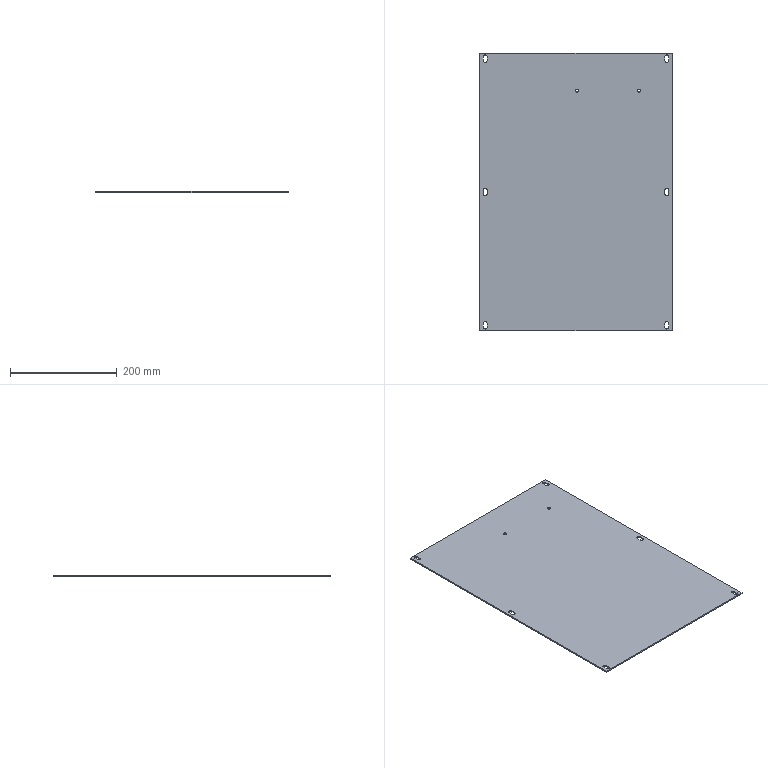Part | SolidWorks | features FlatPattern 1, SMBaseFlange 1, SheetMetal 1 | 1 solid | 34 faces | box 360 x 520 x 2.5 mm | volume 466582 mm3 | plane 18 | cylinder 16 | commonest cylinder face diameters 7 x12 5.2 x4
STEP:
#1=CARTESIAN_POINT('',(-180.6,450.,2.5));
#2=VERTEX_POINT('',#1);
#3=CARTESIAN_POINT('',(-175.4,450.,2.5));
#4=VERTEX_POINT('',#3);
#5=CARTESIAN_POINT('',(-178.,450.,2.5));
#6=DIRECTION('',(0.,0.,1.));
#7=DIRECTION('',(1.,0.,0.));
#8=AXIS2_PLACEMENT_3D('',#5,#6,#7);
#9=CIRCLE('',#8,2.6);
#10=EDGE_CURVE('',#2,#4,#9,.T.);
#11=ORIENTED_EDGE('',*,*,#10,.T.);
#12=CARTESIAN_POINT('',(-175.4,450.,0.));
#13=VERTEX_POINT('',#12);
#14=CARTESIAN_POINT('',(-175.4,450.,2.5));
#15=DIRECTION('',(0.,0.,-1.));
#16=VECTOR('',#15,1000.);
#17=LINE('',#14,#16);
#18=EDGE_CURVE('',#4,#13,#17,.T.);
#19=ORIENTED_EDGE('',*,*,#18,.T.);
#20=CARTESIAN_POINT('',(-180.6,450.,0.));
#21=VERTEX_POINT('',#20);
#22=CARTESIAN_POINT('',(-178.,450.,0.));
#23=DIRECTION('',(0.,0.,1.));
#24=DIRECTION('',(1.,0.,0.));
#25=AXIS2_PLACEMENT_3D('',#22,#23,#24);
#26=CIRCLE('',#25,2.6);
#27=EDGE_CURVE('',#21,#13,#26,.T.);
#28=ORIENTED_EDGE('',*,*,#27,.F.);
#29=CARTESIAN_POINT('',(-180.6,450.,2.5));
#30=DIRECTION('',(0.,0.,-1.));
#31=VECTOR('',#30,1000.);
#32=LINE('',#29,#31);
#33=EDGE_CURVE('',#2,#21,#32,.T.);
#34=ORIENTED_EDGE('',*,*,#33,.F.);
#35=EDGE_LOOP('',(#11,#19,#28,#34));
#36=FACE_OUTER_BOUND('',#35,.T.);
#37=CARTESIAN_POINT('',(-178.,450.,2.5));
#38=DIRECTION('',(0.,0.,-1.));
#39=DIRECTION('',(-1.,0.,0.));
#40=AXIS2_PLACEMENT_3D('',#37,#38,#39);
#41=CYLINDRICAL_SURFACE('',#40,2.6);
#42=ADVANCED_FACE('',(#36),#41,.F.);
#43=CARTESIAN_POINT('',(-64.6,450.,2.5));
#44=VERTEX_POINT('',#43);
#45=CARTESIAN_POINT('',(-59.4,450.,2.5));
#46=VERTEX_POINT('',#45);
#47=CARTESIAN_POINT('',(-62.,450.,2.5));
#48=DIRECTION('',(0.,0.,1.));
#49=DIRECTION('',(1.,0.,0.));
#50=AXIS2_PLACEMENT_3D('',#47,#48,#49);
#51=CIRCLE('',#50,2.6);
#52=EDGE_CURVE('',#44,#46,#51,.T.);
#53=ORIENTED_EDGE('',*,*,#52,.T.);
#54=CARTESIAN_POINT('',(-59.4,450.,0.));
#55=VERTEX_POINT('',#54);
#56=CARTESIAN_POINT('',(-59.4,450.,2.5));
#57=DIRECTION('',(0.,0.,-1.));
#58=VECTOR('',#57,1000.);
#59=LINE('',#56,#58);
#60=EDGE_CURVE('',#46,#55,#59,.T.);
#61=ORIENTED_EDGE('',*,*,#60,.T.);
#62=CARTESIAN_POINT('',(-64.6,450.,0.));
#63=VERTEX_POINT('',#62);
#64=CARTESIAN_POINT('',(-62.,450.,0.));
#65=DIRECTION('',(0.,0.,1.));
#66=DIRECTION('',(1.,0.,0.));
#67=AXIS2_PLACEMENT_3D('',#64,#65,#66);
#68=CIRCLE('',#67,2.6);
#69=EDGE_CURVE('',#63,#55,#68,.T.);
#70=ORIENTED_EDGE('',*,*,#69,.F.);
#71=CARTESIAN_POINT('',(-64.6,450.,2.5));
#72=DIRECTION('',(0.,0.,-1.));
#73=VECTOR('',#72,1000.);
#74=LINE('',#71,#73);
#75=EDGE_CURVE('',#44,#63,#74,.T.);
#76=ORIENTED_EDGE('',*,*,#75,.F.);
#77=EDGE_LOOP('',(#53,#61,#70,#76));
#78=FACE_OUTER_BOUND('',#77,.T.);
#79=CARTESIAN_POINT('',(-62.,450.,2.5));
#80=DIRECTION('',(0.,0.,-1.));
#81=DIRECTION('',(-1.,0.,0.));
#82=AXIS2_PLACEMENT_3D('',#79,#80,#81);
#83=CYLINDRICAL_SURFACE('',#82,2.6);
#84=ADVANCED_FACE('',(#78),#83,.F.);
#85=CARTESIAN_POINT('',(-13.5,513.5,2.5));
#86=VERTEX_POINT('',#85);
#87=CARTESIAN_POINT('',(-13.5,506.5,2.5));
#88=VERTEX_POINT('',#87);
#89=CARTESIAN_POINT('',(-13.5,513.5,2.5));
#90=DIRECTION('',(0.,-1.,0.));
#91=VECTOR('',#90,1000.);
#92=LINE('',#89,#91);
#93=EDGE_CURVE('',#86,#88,#92,.T.);
#94=ORIENTED_EDGE('',*,*,#93,.F.);
#95=CARTESIAN_POINT('',(-6.5,513.5,2.5));
#96=VERTEX_POINT('',#95);
#97=CARTESIAN_POINT('',(-10.,513.5,2.5));
#98=DIRECTION('',(0.,0.,1.));
#99=DIRECTION('',(-1.,0.,0.));
#100=AXIS2_PLACEMENT_3D('',#97,#98,#99);
#101=CIRCLE('',#100,3.5);
#102=EDGE_CURVE('',#96,#86,#101,.T.);
#103=ORIENTED_EDGE('',*,*,#102,.F.);
#104=CARTESIAN_POINT('',(-6.5,506.5,2.5));
#105=VERTEX_POINT('',#104);
#106=CARTESIAN_POINT('',(-6.5,513.5,2.5));
#107=DIRECTION('',(0.,1.,0.));
#108=VECTOR('',#107,1000.);
#109=LINE('',#106,#108);
#110=EDGE_CURVE('',#105,#96,#109,.T.);
#111=ORIENTED_EDGE('',*,*,#110,.F.);
#112=CARTESIAN_POINT('',(-10.,506.5,2.5));
#113=DIRECTION('',(0.,0.,1.));
#114=DIRECTION('',(-1.,0.,0.));
#115=AXIS2_PLACEMENT_3D('',#112,#113,#114);
#116=CIRCLE('',#115,3.5);
#117=EDGE_CURVE('',#88,#105,#116,.T.);
#118=ORIENTED_EDGE('',*,*,#117,.F.);
#119=EDGE_LOOP('',(#94,#103,#111,#118));
#120=FACE_BOUND('',#119,.T.);
#121=CARTESIAN_POINT('',(-13.5,263.5,2.5));
#122=VERTEX_POINT('',#121);
#123=CARTESIAN_POINT('',(-13.5,256.5,2.5));
#124=VERTEX_POINT('',#123);
#125=CARTESIAN_POINT('',(-13.5,263.5,2.5));
#126=DIRECTION('',(0.,-1.,0.));
#127=VECTOR('',#126,1000.);
#128=LINE('',#125,#127);
#129=EDGE_CURVE('',#122,#124,#128,.T.);
#130=ORIENTED_EDGE('',*,*,#129,.F.);
#131=CARTESIAN_POINT('',(-6.5,263.5,2.5));
#132=VERTEX_POINT('',#131);
#133=CARTESIAN_POINT('',(-10.,263.5,2.5));
#134=DIRECTION('',(0.,0.,1.));
#135=DIRECTION('',(-1.,0.,0.));
#136=AXIS2_PLACEMENT_3D('',#133,#134,#135);
#137=CIRCLE('',#136,3.5);
#138=EDGE_CURVE('',#132,#122,#137,.T.);
#139=ORIENTED_EDGE('',*,*,#138,.F.);
#140=CARTESIAN_POINT('',(-6.5,256.5,2.5));
#141=VERTEX_POINT('',#140);
#142=CARTESIAN_POINT('',(-6.5,263.5,2.5));
#143=DIRECTION('',(0.,1.,0.));
#144=VECTOR('',#143,1000.);
#145=LINE('',#142,#144);
#146=EDGE_CURVE('',#141,#132,#145,.T.);
#147=ORIENTED_EDGE('',*,*,#146,.F.);
#148=CARTESIAN_POINT('',(-10.,256.5,2.5));
#149=DIRECTION('',(0.,0.,1.));
#150=DIRECTION('',(-1.,0.,0.));
#151=AXIS2_PLACEMENT_3D('',#148,#149,#150);
#152=CIRCLE('',#151,3.5);
#153=EDGE_CURVE('',#124,#141,#152,.T.);
#154=ORIENTED_EDGE('',*,*,#153,.F.);
#155=EDGE_LOOP('',(#130,#139,#147,#154));
#156=FACE_BOUND('',#155,.T.);
#157=CARTESIAN_POINT('',(-13.5,13.5,2.5));
#158=VERTEX_POINT('',#157);
#159=CARTESIAN_POINT('',(-13.5,6.5,2.5));
#160=VERTEX_POINT('',#159);
#161=CARTESIAN_POINT('',(-13.5,13.5,2.5));
#162=DIRECTION('',(0.,-1.,0.));
#163=VECTOR('',#162,1000.);
#164=LINE('',#161,#163);
#165=EDGE_CURVE('',#158,#160,#164,.T.);
#166=ORIENTED_EDGE('',*,*,#165,.F.);
#167=CARTESIAN_POINT('',(-6.5,13.5,2.5));
#168=VERTEX_POINT('',#167);
#169=CARTESIAN_POINT('',(-10.,13.5,2.5));
#170=DIRECTION('',(0.,0.,1.));
#171=DIRECTION('',(-1.,0.,0.));
#172=AXIS2_PLACEMENT_3D('',#169,#170,#171);
#173=CIRCLE('',#172,3.5);
#174=EDGE_CURVE('',#168,#158,#173,.T.);
#175=ORIENTED_EDGE('',*,*,#174,.F.);
#176=CARTESIAN_POINT('',(-6.5,6.5,2.5));
#177=VERTEX_POINT('',#176);
#178=CARTESIAN_POINT('',(-6.5,13.5,2.5));
#179=DIRECTION('',(0.,1.,0.));
#180=VECTOR('',#179,1000.);
#181=LINE('',#178,#180);
#182=EDGE_CURVE('',#177,#168,#181,.T.);
#183=ORIENTED_EDGE('',*,*,#182,.F.);
#184=CARTESIAN_POINT('',(-10.,6.5,2.5));
#185=DIRECTION('',(0.,0.,1.));
#186=DIRECTION('',(-1.,0.,0.));
#187=AXIS2_PLACEMENT_3D('',#184,#185,#186);
#188=CIRCLE('',#187,3.5);
#189=EDGE_CURVE('',#160,#177,#188,.T.);
#190=ORIENTED_EDGE('',*,*,#189,.F.);
#191=EDGE_LOOP('',(#166,#175,#183,#190));
#192=FACE_BOUND('',#191,.T.);
#193=CARTESIAN_POINT('',(-353.5,13.5,2.5));
#194=VERTEX_POINT('',#193);
#195=CARTESIAN_POINT('',(-353.5,6.5,2.5));
#196=VERTEX_POINT('',#195);
#197=CARTESIAN_POINT('',(-353.5,13.5,2.5));
#198=DIRECTION('',(0.,-1.,0.));
#199=VECTOR('',#198,1000.);
#200=LINE('',#197,#199);
#201=EDGE_CURVE('',#194,#196,#200,.T.);
#202=ORIENTED_EDGE('',*,*,#201,.F.);
#203=CARTESIAN_POINT('',(-346.5,13.5,2.5));
#204=VERTEX_POINT('',#203);
#205=CARTESIAN_POINT('',(-350.,13.5,2.5));
#206=DIRECTION('',(0.,0.,1.));
#207=DIRECTION('',(-1.,0.,0.));
#208=AXIS2_PLACEMENT_3D('',#205,#206,#207);
#209=CIRCLE('',#208,3.5);
#210=EDGE_CURVE('',#204,#194,#209,.T.);
#211=ORIENTED_EDGE('',*,*,#210,.F.);
#212=CARTESIAN_POINT('',(-346.5,6.5,2.5));
#213=VERTEX_POINT('',#212);
#214=CARTESIAN_POINT('',(-346.5,13.5,2.5));
#215=DIRECTION('',(0.,1.,0.));
#216=VECTOR('',#215,1000.);
#217=LINE('',#214,#216);
#218=EDGE_CURVE('',#213,#204,#217,.T.);
#219=ORIENTED_EDGE('',*,*,#218,.F.);
#220=CARTESIAN_POINT('',(-350.,6.5,2.5));
#221=DIRECTION('',(0.,0.,1.));
#222=DIRECTION('',(-1.,0.,0.));
#223=AXIS2_PLACEMENT_3D('',#220,#221,#222);
#224=CIRCLE('',#223,3.5);
#225=EDGE_CURVE('',#196,#213,#224,.T.);
#226=ORIENTED_EDGE('',*,*,#225,.F.);
#227=EDGE_LOOP('',(#202,#211,#219,#226));
#228=FACE_BOUND('',#227,.T.);
#229=CARTESIAN_POINT('',(0.,0.,2.5));
#230=VERTEX_POINT('',#229);
#231=CARTESIAN_POINT('',(0.,520.,2.5));
#232=VERTEX_POINT('',#231);
#233=CARTESIAN_POINT('',(0.,0.,2.5));
#234=DIRECTION('',(0.,1.,0.));
#235=VECTOR('',#234,1000.);
#236=LINE('',#233,#235);
#237=EDGE_CURVE('',#230,#232,#236,.T.);
#238=ORIENTED_EDGE('',*,*,#237,.T.);
#239=CARTESIAN_POINT('',(-360.,520.,2.5));
#240=VERTEX_POINT('',#239);
#241=CARTESIAN_POINT('',(0.,520.,2.5));
#242=DIRECTION('',(-1.,0.,0.));
#243=VECTOR('',#242,1000.);
#244=LINE('',#241,#243);
#245=EDGE_CURVE('',#232,#240,#244,.T.);
#246=ORIENTED_EDGE('',*,*,#245,.T.);
#247=CARTESIAN_POINT('',(-360.,0.,2.5));
#248=VERTEX_POINT('',#247);
#249=CARTESIAN_POINT('',(-360.,0.,2.5));
#250=DIRECTION('',(0.,-1.,0.));
#251=VECTOR('',#250,1000.);
#252=LINE('',#249,#251);
#253=EDGE_CURVE('',#240,#248,#252,.T.);
#254=ORIENTED_EDGE('',*,*,#253,.T.);
#255=CARTESIAN_POINT('',(0.,0.,2.5));
#256=DIRECTION('',(1.,0.,0.));
#257=VECTOR('',#256,1000.);
#258=LINE('',#255,#257);
#259=EDGE_CURVE('',#248,#230,#258,.T.);
#260=ORIENTED_EDGE('',*,*,#259,.T.);
#261=EDGE_LOOP('',(#238,#246,#254,#260));
#262=FACE_OUTER_BOUND('',#261,.T.);
#263=ORIENTED_EDGE('',*,*,#52,.F.);
#264=CARTESIAN_POINT('',(-62.,450.,2.5));
#265=DIRECTION('',(0.,0.,1.));
#266=DIRECTION('',(1.,0.,0.));
#267=AXIS2_PLACEMENT_3D('',#264,#265,#266);
#268=CIRCLE('',#267,2.6);
#269=EDGE_CURVE('',#46,#44,#268,.T.);
#270=ORIENTED_EDGE('',*,*,#269,.F.);
#271=EDGE_LOOP('',(#263,#270));
#272=FACE_BOUND('',#271,.T.);
#273=CARTESIAN_POINT('',(-353.5,263.5,2.5));
#274=VERTEX_POINT('',#273);
#275=CARTESIAN_POINT('',(-353.5,256.5,2.5));
#276=VERTEX_POINT('',#275);
#277=CARTESIAN_POINT('',(-353.5,263.5,2.5));
#278=DIRECTION('',(0.,-1.,0.));
#279=VECTOR('',#278,1000.);
#280=LINE('',#277,#279);
#281=EDGE_CURVE('',#274,#276,#280,.T.);
#282=ORIENTED_EDGE('',*,*,#281,.F.);
#283=CARTESIAN_POINT('',(-346.5,263.5,2.5));
#284=VERTEX_POINT('',#283);
#285=CARTESIAN_POINT('',(-350.,263.5,2.5));
#286=DIRECTION('',(0.,0.,1.));
#287=DIRECTION('',(-1.,0.,0.));
#288=AXIS2_PLACEMENT_3D('',#285,#286,#287);
#289=CIRCLE('',#288,3.5);
#290=EDGE_CURVE('',#284,#274,#289,.T.);
#291=ORIENTED_EDGE('',*,*,#290,.F.);
#292=CARTESIAN_POINT('',(-346.5,256.5,2.5));
#293=VERTEX_POINT('',#292);
#294=CARTESIAN_POINT('',(-346.5,263.5,2.5));
#295=DIRECTION('',(0.,1.,0.));
#296=VECTOR('',#295,1000.);
#297=LINE('',#294,#296);
#298=EDGE_CURVE('',#293,#284,#297,.T.);
#299=ORIENTED_EDGE('',*,*,#298,.F.);
#300=CARTESIAN_POINT('',(-350.,256.5,2.5));
#301=DIRECTION('',(0.,0.,1.));
#302=DIRECTION('',(-1.,0.,0.));
#303=AXIS2_PLACEMENT_3D('',#300,#301,#302);
#304=CIRCLE('',#303,3.5);
#305=EDGE_CURVE('',#276,#293,#304,.T.);
#306=ORIENTED_EDGE('',*,*,#305,.F.);
#307=EDGE_LOOP('',(#282,#291,#299,#306));
#308=FACE_BOUND('',#307,.T.);
#309=CARTESIAN_POINT('',(-353.5,513.5,2.5));
#310=VERTEX_POINT('',#309);
#311=CARTESIAN_POINT('',(-353.5,506.5,2.5));
#312=VERTEX_POINT('',#311);
#313=CARTESIAN_POINT('',(-353.5,513.5,2.5));
#314=DIRECTION('',(0.,-1.,0.));
#315=VECTOR('',#314,1000.);
#316=LINE('',#313,#315);
#317=EDGE_CURVE('',#310,#312,#316,.T.);
#318=ORIENTED_EDGE('',*,*,#317,.F.);
#319=CARTESIAN_POINT('',(-346.5,513.5,2.5));
#320=VERTEX_POINT('',#319);
#321=CARTESIAN_POINT('',(-350.,513.5,2.5));
#322=DIRECTION('',(0.,0.,1.));
#323=DIRECTION('',(-1.,0.,0.));
#324=AXIS2_PLACEMENT_3D('',#321,#322,#323);
#325=CIRCLE('',#324,3.5);
#326=EDGE_CURVE('',#320,#310,#325,.T.);
#327=ORIENTED_EDGE('',*,*,#326,.F.);
#328=CARTESIAN_POINT('',(-346.5,506.5,2.5));
#329=VERTEX_POINT('',#328);
#330=CARTESIAN_POINT('',(-346.5,513.5,2.5));
#331=DIRECTION('',(0.,1.,0.));
#332=VECTOR('',#331,1000.);
#333=LINE('',#330,#332);
#334=EDGE_CURVE('',#329,#320,#333,.T.);
#335=ORIENTED_EDGE('',*,*,#334,.F.);
#336=CARTESIAN_POINT('',(-350.,506.5,2.5));
#337=DIRECTION('',(0.,0.,1.));
#338=DIRECTION('',(-1.,0.,0.));
#339=AXIS2_PLACEMENT_3D('',#336,#337,#338);
#340=CIRCLE('',#339,3.5);
#341=EDGE_CURVE('',#312,#329,#340,.T.);
#342=ORIENTED_EDGE('',*,*,#341,.F.);
#343=EDGE_LOOP('',(#318,#327,#335,#342));
#344=FACE_BOUND('',#343,.T.);
#345=ORIENTED_EDGE('',*,*,#10,.F.);
#346=CARTESIAN_POINT('',(-178.,450.,2.5));
#347=DIRECTION('',(0.,0.,1.));
#348=DIRECTION('',(1.,0.,0.));
#349=AXIS2_PLACEMENT_3D('',#346,#347,#348);
#350=CIRCLE('',#349,2.6);
#351=EDGE_CURVE('',#4,#2,#350,.T.);
#352=ORIENTED_EDGE('',*,*,#351,.F.);
#353=EDGE_LOOP('',(#345,#352));
#354=FACE_BOUND('',#353,.T.);
#355=CARTESIAN_POINT('',(0.,0.,2.5));
#356=DIRECTION('',(0.,0.,1.));
#357=DIRECTION('',(1.,0.,0.));
#358=AXIS2_PLACEMENT_3D('',#355,#356,#357);
#359=PLANE('',#358);
#360=ADVANCED_FACE('',(#120,#156,#192,#228,#262,#272,#308,#344,#354),#359,.T.);
#361=CARTESIAN_POINT('',(-6.5,513.5,0.));
#362=VERTEX_POINT('',#361);
#363=CARTESIAN_POINT('',(-13.5,513.5,0.));
#364=VERTEX_POINT('',#363);
#365=CARTESIAN_POINT('',(-10.,513.5,0.));
#366=DIRECTION('',(0.,0.,1.));
#367=DIRECTION('',(-1.,0.,0.));
#368=AXIS2_PLACEMENT_3D('',#365,#366,#367);
#369=CIRCLE('',#368,3.5);
#370=EDGE_CURVE('',#362,#364,#369,.T.);
#371=ORIENTED_EDGE('',*,*,#370,.T.);
#372=CARTESIAN_POINT('',(-13.5,506.5,0.));
#373=VERTEX_POINT('',#372);
#374=CARTESIAN_POINT('',(-13.5,513.5,0.));
#375=DIRECTION('',(0.,-1.,0.));
#376=VECTOR('',#375,1000.);
#377=LINE('',#374,#376);
#378=EDGE_CURVE('',#364,#373,#377,.T.);
#379=ORIENTED_EDGE('',*,*,#378,.T.);
#380=CARTESIAN_POINT('',(-6.5,506.5,0.));
#381=VERTEX_POINT('',#380);
#382=CARTESIAN_POINT('',(-10.,506.5,0.));
#383=DIRECTION('',(0.,0.,1.));
#384=DIRECTION('',(-1.,0.,0.));
#385=AXIS2_PLACEMENT_3D('',#382,#383,#384);
#386=CIRCLE('',#385,3.5);
#387=EDGE_CURVE('',#373,#381,#386,.T.);
#388=ORIENTED_EDGE('',*,*,#387,.T.);
#389=CARTESIAN_POINT('',(-6.5,513.5,0.));
#390=DIRECTION('',(0.,1.,0.));
#391=VECTOR('',#390,1000.);
#392=LINE('',#389,#391);
#393=EDGE_CURVE('',#381,#362,#392,.T.);
#394=ORIENTED_EDGE('',*,*,#393,.T.);
#395=EDGE_LOOP('',(#371,#379,#388,#394));
#396=FACE_BOUND('',#395,.T.);
#397=CARTESIAN_POINT('',(-6.5,263.5,0.));
#398=VERTEX_POINT('',#397);
#399=CARTESIAN_POINT('',(-13.5,263.5,0.));
#400=VERTEX_POINT('',#399);
#401=CARTESIAN_POINT('',(-10.,263.5,0.));
#402=DIRECTION('',(0.,0.,1.));
#403=DIRECTION('',(-1.,0.,0.));
#404=AXIS2_PLACEMENT_3D('',#401,#402,#403);
#405=CIRCLE('',#404,3.5);
#406=EDGE_CURVE('',#398,#400,#405,.T.);
#407=ORIENTED_EDGE('',*,*,#406,.T.);
#408=CARTESIAN_POINT('',(-13.5,256.5,0.));
#409=VERTEX_POINT('',#408);
#410=CARTESIAN_POINT('',(-13.5,263.5,0.));
#411=DIRECTION('',(0.,-1.,0.));
#412=VECTOR('',#411,1000.);
#413=LINE('',#410,#412);
#414=EDGE_CURVE('',#400,#409,#413,.T.);
#415=ORIENTED_EDGE('',*,*,#414,.T.);
#416=CARTESIAN_POINT('',(-6.5,256.5,0.));
#417=VERTEX_POINT('',#416);
#418=CARTESIAN_POINT('',(-10.,256.5,0.));
#419=DIRECTION('',(0.,0.,1.));
#420=DIRECTION('',(-1.,0.,0.));
#421=AXIS2_PLACEMENT_3D('',#418,#419,#420);
#422=CIRCLE('',#421,3.5);
#423=EDGE_CURVE('',#409,#417,#422,.T.);
#424=ORIENTED_EDGE('',*,*,#423,.T.);
#425=CARTESIAN_POINT('',(-6.5,263.5,0.));
#426=DIRECTION('',(0.,1.,0.));
#427=VECTOR('',#426,1000.);
#428=LINE('',#425,#427);
#429=EDGE_CURVE('',#417,#398,#428,.T.);
#430=ORIENTED_EDGE('',*,*,#429,.T.);
#431=EDGE_LOOP('',(#407,#415,#424,#430));
#432=FACE_BOUND('',#431,.T.);
#433=CARTESIAN_POINT('',(-6.5,13.5,0.));
#434=VERTEX_POINT('',#433);
#435=CARTESIAN_POINT('',(-13.5,13.5,0.));
#436=VERTEX_POINT('',#435);
#437=CARTESIAN_POINT('',(-10.,13.5,0.));
#438=DIRECTION('',(0.,0.,1.));
#439=DIRECTION('',(-1.,0.,0.));
#440=AXIS2_PLACEMENT_3D('',#437,#438,#439);
#441=CIRCLE('',#440,3.5);
#442=EDGE_CURVE('',#434,#436,#441,.T.);
#443=ORIENTED_EDGE('',*,*,#442,.T.);
#444=CARTESIAN_POINT('',(-13.5,6.5,0.));
#445=VERTEX_POINT('',#444);
#446=CARTESIAN_POINT('',(-13.5,13.5,0.));
#447=DIRECTION('',(0.,-1.,0.));
#448=VECTOR('',#447,1000.);
#449=LINE('',#446,#448);
#450=EDGE_CURVE('',#436,#445,#449,.T.);
#451=ORIENTED_EDGE('',*,*,#450,.T.);
#452=CARTESIAN_POINT('',(-6.5,6.5,0.));
#453=VERTEX_POINT('',#452);
#454=CARTESIAN_POINT('',(-10.,6.5,0.));
#455=DIRECTION('',(0.,0.,1.));
#456=DIRECTION('',(-1.,0.,0.));
#457=AXIS2_PLACEMENT_3D('',#454,#455,#456);
#458=CIRCLE('',#457,3.5);
#459=EDGE_CURVE('',#445,#453,#458,.T.);
#460=ORIENTED_EDGE('',*,*,#459,.T.);
#461=CARTESIAN_POINT('',(-6.5,13.5,0.));
#462=DIRECTION('',(0.,1.,0.));
#463=VECTOR('',#462,1000.);
#464=LINE('',#461,#463);
#465=EDGE_CURVE('',#453,#434,#464,.T.);
#466=ORIENTED_EDGE('',*,*,#465,.T.);
#467=EDGE_LOOP('',(#443,#451,#460,#466));
#468=FACE_BOUND('',#467,.T.);
#469=CARTESIAN_POINT('',(-346.5,13.5,0.));
#470=VERTEX_POINT('',#469);
#471=CARTESIAN_POINT('',(-353.5,13.5,0.));
#472=VERTEX_POINT('',#471);
#473=CARTESIAN_POINT('',(-350.,13.5,0.));
#474=DIRECTION('',(0.,0.,1.));
#475=DIRECTION('',(-1.,0.,0.));
#476=AXIS2_PLACEMENT_3D('',#473,#474,#475);
#477=CIRCLE('',#476,3.5);
#478=EDGE_CURVE('',#470,#472,#477,.T.);
#479=ORIENTED_EDGE('',*,*,#478,.T.);
#480=CARTESIAN_POINT('',(-353.5,6.5,0.));
#481=VERTEX_POINT('',#480);
#482=CARTESIAN_POINT('',(-353.5,13.5,0.));
#483=DIRECTION('',(0.,-1.,0.));
#484=VECTOR('',#483,1000.);
#485=LINE('',#482,#484);
#486=EDGE_CURVE('',#472,#481,#485,.T.);
#487=ORIENTED_EDGE('',*,*,#486,.T.);
#488=CARTESIAN_POINT('',(-346.5,6.5,0.));
#489=VERTEX_POINT('',#488);
#490=CARTESIAN_POINT('',(-350.,6.5,0.));
#491=DIRECTION('',(0.,0.,1.));
#492=DIRECTION('',(-1.,0.,0.));
#493=AXIS2_PLACEMENT_3D('',#490,#491,#492);
#494=CIRCLE('',#493,3.5);
#495=EDGE_CURVE('',#481,#489,#494,.T.);
#496=ORIENTED_EDGE('',*,*,#495,.T.);
#497=CARTESIAN_POINT('',(-346.5,13.5,0.));
#498=DIRECTION('',(0.,1.,0.));
#499=VECTOR('',#498,1000.);
#500=LINE('',#497,#499);
#501=EDGE_CURVE('',#489,#470,#500,.T.);
#502=ORIENTED_EDGE('',*,*,#501,.T.);
#503=EDGE_LOOP('',(#479,#487,#496,#502));
#504=FACE_BOUND('',#503,.T.);
#505=CARTESIAN_POINT('',(0.,0.,0.));
#506=VERTEX_POINT('',#505);
#507=CARTESIAN_POINT('',(0.,520.,0.));
#508=VERTEX_POINT('',#507);
#509=CARTESIAN_POINT('',(0.,0.,0.));
#510=DIRECTION('',(0.,1.,0.));
#511=VECTOR('',#510,1000.);
#512=LINE('',#509,#511);
#513=EDGE_CURVE('',#506,#508,#512,.T.);
#514=ORIENTED_EDGE('',*,*,#513,.F.);
#515=CARTESIAN_POINT('',(-360.,0.,0.));
#516=VERTEX_POINT('',#515);
#517=CARTESIAN_POINT('',(0.,0.,0.));
#518=DIRECTION('',(1.,0.,0.));
#519=VECTOR('',#518,1000.);
#520=LINE('',#517,#519);
#521=EDGE_CURVE('',#516,#506,#520,.T.);
#522=ORIENTED_EDGE('',*,*,#521,.F.);
#523=CARTESIAN_POINT('',(-360.,520.,0.));
#524=VERTEX_POINT('',#523);
#525=CARTESIAN_POINT('',(-360.,0.,0.));
#526=DIRECTION('',(0.,-1.,0.));
#527=VECTOR('',#526,1000.);
#528=LINE('',#525,#527);
#529=EDGE_CURVE('',#524,#516,#528,.T.);
#530=ORIENTED_EDGE('',*,*,#529,.F.);
#531=CARTESIAN_POINT('',(0.,520.,0.));
#532=DIRECTION('',(-1.,0.,0.));
#533=VECTOR('',#532,1000.);
#534=LINE('',#531,#533);
#535=EDGE_CURVE('',#508,#524,#534,.T.);
#536=ORIENTED_EDGE('',*,*,#535,.F.);
#537=EDGE_LOOP('',(#514,#522,#530,#536));
#538=FACE_OUTER_BOUND('',#537,.T.);
#539=ORIENTED_EDGE('',*,*,#69,.T.);
#540=CARTESIAN_POINT('',(-62.,450.,0.));
#541=DIRECTION('',(0.,0.,1.));
#542=DIRECTION('',(1.,0.,0.));
#543=AXIS2_PLACEMENT_3D('',#540,#541,#542);
#544=CIRCLE('',#543,2.6);
#545=EDGE_CURVE('',#55,#63,#544,.T.);
#546=ORIENTED_EDGE('',*,*,#545,.T.);
#547=EDGE_LOOP('',(#539,#546));
#548=FACE_BOUND('',#547,.T.);
#549=CARTESIAN_POINT('',(-346.5,263.5,0.));
#550=VERTEX_POINT('',#549);
#551=CARTESIAN_POINT('',(-353.5,263.5,0.));
#552=VERTEX_POINT('',#551);
#553=CARTESIAN_POINT('',(-350.,263.5,0.));
#554=DIRECTION('',(0.,0.,1.));
#555=DIRECTION('',(-1.,0.,0.));
#556=AXIS2_PLACEMENT_3D('',#553,#554,#555);
#557=CIRCLE('',#556,3.5);
#558=EDGE_CURVE('',#550,#552,#557,.T.);
#559=ORIENTED_EDGE('',*,*,#558,.T.);
#560=CARTESIAN_POINT('',(-353.5,256.5,0.));
#561=VERTEX_POINT('',#560);
#562=CARTESIAN_POINT('',(-353.5,263.5,0.));
#563=DIRECTION('',(0.,-1.,0.));
#564=VECTOR('',#563,1000.);
#565=LINE('',#562,#564);
#566=EDGE_CURVE('',#552,#561,#565,.T.);
#567=ORIENTED_EDGE('',*,*,#566,.T.);
#568=CARTESIAN_POINT('',(-346.5,256.5,0.));
#569=VERTEX_POINT('',#568);
#570=CARTESIAN_POINT('',(-350.,256.5,0.));
#571=DIRECTION('',(0.,0.,1.));
#572=DIRECTION('',(-1.,0.,0.));
#573=AXIS2_PLACEMENT_3D('',#570,#571,#572);
#574=CIRCLE('',#573,3.5);
#575=EDGE_CURVE('',#561,#569,#574,.T.);
#576=ORIENTED_EDGE('',*,*,#575,.T.);
#577=CARTESIAN_POINT('',(-346.5,263.5,0.));
#578=DIRECTION('',(0.,1.,0.));
#579=VECTOR('',#578,1000.);
#580=LINE('',#577,#579);
#581=EDGE_CURVE('',#569,#550,#580,.T.);
#582=ORIENTED_EDGE('',*,*,#581,.T.);
#583=EDGE_LOOP('',(#559,#567,#576,#582));
#584=FACE_BOUND('',#583,.T.);
#585=CARTESIAN_POINT('',(-346.5,513.5,0.));
#586=VERTEX_POINT('',#585);
#587=CARTESIAN_POINT('',(-353.5,513.5,0.));
#588=VERTEX_POINT('',#587);
#589=CARTESIAN_POINT('',(-350.,513.5,0.));
#590=DIRECTION('',(0.,0.,1.));
#591=DIRECTION('',(-1.,0.,0.));
#592=AXIS2_PLACEMENT_3D('',#589,#590,#591);
#593=CIRCLE('',#592,3.5);
#594=EDGE_CURVE('',#586,#588,#593,.T.);
#595=ORIENTED_EDGE('',*,*,#594,.T.);
#596=CARTESIAN_POINT('',(-353.5,506.5,0.));
#597=VERTEX_POINT('',#596);
#598=CARTESIAN_POINT('',(-353.5,513.5,0.));
#599=DIRECTION('',(0.,-1.,0.));
#600=VECTOR('',#599,1000.);
#601=LINE('',#598,#600);
#602=EDGE_CURVE('',#588,#597,#601,.T.);
#603=ORIENTED_EDGE('',*,*,#602,.T.);
#604=CARTESIAN_POINT('',(-346.5,506.5,0.));
#605=VERTEX_POINT('',#604);
#606=CARTESIAN_POINT('',(-350.,506.5,0.));
#607=DIRECTION('',(0.,0.,1.));
#608=DIRECTION('',(-1.,0.,0.));
#609=AXIS2_PLACEMENT_3D('',#606,#607,#608);
#610=CIRCLE('',#609,3.5);
#611=EDGE_CURVE('',#597,#605,#610,.T.);
#612=ORIENTED_EDGE('',*,*,#611,.T.);
#613=CARTESIAN_POINT('',(-346.5,513.5,0.));
#614=DIRECTION('',(0.,1.,0.));
#615=VECTOR('',#614,1000.);
#616=LINE('',#613,#615);
#617=EDGE_CURVE('',#605,#586,#616,.T.);
#618=ORIENTED_EDGE('',*,*,#617,.T.);
#619=EDGE_LOOP('',(#595,#603,#612,#618));
#620=FACE_BOUND('',#619,.T.);
#621=ORIENTED_EDGE('',*,*,#27,.T.);
#622=CARTESIAN_POINT('',(-178.,450.,0.));
#623=DIRECTION('',(0.,0.,1.));
#624=DIRECTION('',(1.,0.,0.));
#625=AXIS2_PLACEMENT_3D('',#622,#623,#624);
#626=CIRCLE('',#625,2.6);
#627=EDGE_CURVE('',#13,#21,#626,.T.);
#628=ORIENTED_EDGE('',*,*,#627,.T.);
#629=EDGE_LOOP('',(#621,#628));
#630=FACE_BOUND('',#629,.T.);
#631=CARTESIAN_POINT('',(0.,0.,0.));
#632=DIRECTION('',(0.,0.,1.));
#633=DIRECTION('',(1.,0.,0.));
#634=AXIS2_PLACEMENT_3D('',#631,#632,#633);
#635=PLANE('',#634);
#636=ADVANCED_FACE('',(#396,#432,#468,#504,#538,#548,#584,#620,#630),#635,.F.);
#637=ORIENTED_EDGE('',*,*,#513,.T.);
#638=CARTESIAN_POINT('',(0.,520.,2.5));
#639=DIRECTION('',(0.,0.,-1.));
#640=VECTOR('',#639,1000.);
#641=LINE('',#638,#640);
#642=EDGE_CURVE('',#232,#508,#641,.T.);
#643=ORIENTED_EDGE('',*,*,#642,.F.);
#644=ORIENTED_EDGE('',*,*,#237,.F.);
#645=CARTESIAN_POINT('',(0.,0.,2.5));
#646=DIRECTION('',(0.,0.,-1.));
#647=VECTOR('',#646,1000.);
#648=LINE('',#645,#647);
#649=EDGE_CURVE('',#230,#506,#648,.T.);
#650=ORIENTED_EDGE('',*,*,#649,.T.);
#651=EDGE_LOOP('',(#637,#643,#644,#650));
#652=FACE_OUTER_BOUND('',#651,.T.);
#653=CARTESIAN_POINT('',(0.,0.,2.5));
#654=DIRECTION('',(-1.,0.,0.));
#655=DIRECTION('',(0.,0.,1.));
#656=AXIS2_PLACEMENT_3D('',#653,#654,#655);
#657=PLANE('',#656);
#658=ADVANCED_FACE('',(#652),#657,.F.);
#659=ORIENTED_EDGE('',*,*,#535,.T.);
#660=CARTESIAN_POINT('',(-360.,520.,2.5));
#661=DIRECTION('',(0.,0.,-1.));
#662=VECTOR('',#661,1000.);
#663=LINE('',#660,#662);
#664=EDGE_CURVE('',#240,#524,#663,.T.);
#665=ORIENTED_EDGE('',*,*,#664,.F.);
#666=ORIENTED_EDGE('',*,*,#245,.F.);
#667=ORIENTED_EDGE('',*,*,#642,.T.);
#668=EDGE_LOOP('',(#659,#665,#666,#667));
#669=FACE_OUTER_BOUND('',#668,.T.);
#670=CARTESIAN_POINT('',(0.,520.,2.5));
#671=DIRECTION('',(0.,-1.,0.));
#672=DIRECTION('',(1.,0.,0.));
#673=AXIS2_PLACEMENT_3D('',#670,#671,#672);
#674=PLANE('',#673);
#675=ADVANCED_FACE('',(#669),#674,.F.);
#676=ORIENTED_EDGE('',*,*,#529,.T.);
#677=CARTESIAN_POINT('',(-360.,0.,2.5));
#678=DIRECTION('',(0.,0.,-1.));
#679=VECTOR('',#678,1000.);
#680=LINE('',#677,#679);
#681=EDGE_CURVE('',#248,#516,#680,.T.);
#682=ORIENTED_EDGE('',*,*,#681,.F.);
#683=ORIENTED_EDGE('',*,*,#253,.F.);
#684=ORIENTED_EDGE('',*,*,#664,.T.);
#685=EDGE_LOOP('',(#676,#682,#683,#684));
#686=FACE_OUTER_BOUND('',#685,.T.);
#687=CARTESIAN_POINT('',(-360.,0.,2.5));
#688=DIRECTION('',(1.,0.,0.));
#689=DIRECTION('',(0.,0.,-1.));
#690=AXIS2_PLACEMENT_3D('',#687,#688,#689);
#691=PLANE('',#690);
#692=ADVANCED_FACE('',(#686),#691,.F.);
#693=ORIENTED_EDGE('',*,*,#521,.T.);
#694=ORIENTED_EDGE('',*,*,#649,.F.);
#695=ORIENTED_EDGE('',*,*,#259,.F.);
#696=ORIENTED_EDGE('',*,*,#681,.T.);
#697=EDGE_LOOP('',(#693,#694,#695,#696));
#698=FACE_OUTER_BOUND('',#697,.T.);
#699=CARTESIAN_POINT('',(0.,0.,2.5));
#700=DIRECTION('',(0.,1.,0.));
#701=DIRECTION('',(-1.,0.,0.));
#702=AXIS2_PLACEMENT_3D('',#699,#700,#701);
#703=PLANE('',#702);
#704=ADVANCED_FACE('',(#698),#703,.F.);
#705=ORIENTED_EDGE('',*,*,#478,.F.);
#706=CARTESIAN_POINT('',(-346.5,13.5,2.5));
#707=DIRECTION('',(0.,0.,-1.));
#708=VECTOR('',#707,1000.);
#709=LINE('',#706,#708);
#710=EDGE_CURVE('',#204,#470,#709,.T.);
#711=ORIENTED_EDGE('',*,*,#710,.F.);
#712=ORIENTED_EDGE('',*,*,#210,.T.);
#713=CARTESIAN_POINT('',(-353.5,13.5,2.5));
#714=DIRECTION('',(0.,0.,-1.));
#715=VECTOR('',#714,1000.);
#716=LINE('',#713,#715);
#717=EDGE_CURVE('',#194,#472,#716,.T.);
#718=ORIENTED_EDGE('',*,*,#717,.T.);
#719=EDGE_LOOP('',(#705,#711,#712,#718));
#720=FACE_OUTER_BOUND('',#719,.T.);
#721=CARTESIAN_POINT('',(-350.,13.5,2.5));
#722=DIRECTION('',(0.,0.,-1.));
#723=DIRECTION('',(-1.,0.,0.));
#724=AXIS2_PLACEMENT_3D('',#721,#722,#723);
#725=CYLINDRICAL_SURFACE('',#724,3.5);
#726=ADVANCED_FACE('',(#720),#725,.F.);
#727=ORIENTED_EDGE('',*,*,#486,.F.);
#728=ORIENTED_EDGE('',*,*,#717,.F.);
#729=ORIENTED_EDGE('',*,*,#201,.T.);
#730=CARTESIAN_POINT('',(-353.5,6.5,2.5));
#731=DIRECTION('',(0.,0.,-1.));
#732=VECTOR('',#731,1000.);
#733=LINE('',#730,#732);
#734=EDGE_CURVE('',#196,#481,#733,.T.);
#735=ORIENTED_EDGE('',*,*,#734,.T.);
#736=EDGE_LOOP('',(#727,#728,#729,#735));
#737=FACE_OUTER_BOUND('',#736,.T.);
#738=CARTESIAN_POINT('',(-353.5,13.5,2.5));
#739=DIRECTION('',(1.,0.,0.));
#740=DIRECTION('',(0.,0.,-1.));
#741=AXIS2_PLACEMENT_3D('',#738,#739,#740);
#742=PLANE('',#741);
#743=ADVANCED_FACE('',(#737),#742,.T.);
#744=ORIENTED_EDGE('',*,*,#495,.F.);
#745=ORIENTED_EDGE('',*,*,#734,.F.);
#746=ORIENTED_EDGE('',*,*,#225,.T.);
#747=CARTESIAN_POINT('',(-346.5,6.5,2.5));
#748=DIRECTION('',(0.,0.,-1.));
#749=VECTOR('',#748,1000.);
#750=LINE('',#747,#749);
#751=EDGE_CURVE('',#213,#489,#750,.T.);
#752=ORIENTED_EDGE('',*,*,#751,.T.);
#753=EDGE_LOOP('',(#744,#745,#746,#752));
#754=FACE_OUTER_BOUND('',#753,.T.);
#755=CARTESIAN_POINT('',(-350.,6.5,2.5));
#756=DIRECTION('',(0.,0.,-1.));
#757=DIRECTION('',(-1.,0.,0.));
#758=AXIS2_PLACEMENT_3D('',#755,#756,#757);
#759=CYLINDRICAL_SURFACE('',#758,3.5);
#760=ADVANCED_FACE('',(#754),#759,.F.);
#761=ORIENTED_EDGE('',*,*,#501,.F.);
#762=ORIENTED_EDGE('',*,*,#751,.F.);
#763=ORIENTED_EDGE('',*,*,#218,.T.);
#764=ORIENTED_EDGE('',*,*,#710,.T.);
#765=EDGE_LOOP('',(#761,#762,#763,#764));
#766=FACE_OUTER_BOUND('',#765,.T.);
#767=CARTESIAN_POINT('',(-346.5,13.5,2.5));
#768=DIRECTION('',(-1.,0.,0.));
#769=DIRECTION('',(0.,0.,1.));
#770=AXIS2_PLACEMENT_3D('',#767,#768,#769);
#771=PLANE('',#770);
#772=ADVANCED_FACE('',(#766),#771,.T.);
#773=ORIENTED_EDGE('',*,*,#60,.F.);
#774=ORIENTED_EDGE('',*,*,#269,.T.);
#775=ORIENTED_EDGE('',*,*,#75,.T.);
#776=ORIENTED_EDGE('',*,*,#545,.F.);
#777=EDGE_LOOP('',(#773,#774,#775,#776));
#778=FACE_OUTER_BOUND('',#777,.T.);
#779=CARTESIAN_POINT('',(-62.,450.,2.5));
#780=DIRECTION('',(0.,0.,-1.));
#781=DIRECTION('',(-1.,0.,0.));
#782=AXIS2_PLACEMENT_3D('',#779,#780,#781);
#783=CYLINDRICAL_SURFACE('',#782,2.6);
#784=ADVANCED_FACE('',(#778),#783,.F.);
#785=ORIENTED_EDGE('',*,*,#442,.F.);
#786=CARTESIAN_POINT('',(-6.5,13.5,2.5));
#787=DIRECTION('',(0.,0.,-1.));
#788=VECTOR('',#787,1000.);
#789=LINE('',#786,#788);
#790=EDGE_CURVE('',#168,#434,#789,.T.);
#791=ORIENTED_EDGE('',*,*,#790,.F.);
#792=ORIENTED_EDGE('',*,*,#174,.T.);
#793=CARTESIAN_POINT('',(-13.5,13.5,2.5));
#794=DIRECTION('',(0.,0.,-1.));
#795=VECTOR('',#794,1000.);
#796=LINE('',#793,#795);
#797=EDGE_CURVE('',#158,#436,#796,.T.);
#798=ORIENTED_EDGE('',*,*,#797,.T.);
#799=EDGE_LOOP('',(#785,#791,#792,#798));
#800=FACE_OUTER_BOUND('',#799,.T.);
#801=CARTESIAN_POINT('',(-10.,13.5,2.5));
#802=DIRECTION('',(0.,0.,-1.));
#803=DIRECTION('',(-1.,0.,0.));
#804=AXIS2_PLACEMENT_3D('',#801,#802,#803);
#805=CYLINDRICAL_SURFACE('',#804,3.5);
#806=ADVANCED_FACE('',(#800),#805,.F.);
#807=ORIENTED_EDGE('',*,*,#450,.F.);
#808=ORIENTED_EDGE('',*,*,#797,.F.);
#809=ORIENTED_EDGE('',*,*,#165,.T.);
#810=CARTESIAN_POINT('',(-13.5,6.5,2.5));
#811=DIRECTION('',(0.,0.,-1.));
#812=VECTOR('',#811,1000.);
#813=LINE('',#810,#812);
#814=EDGE_CURVE('',#160,#445,#813,.T.);
#815=ORIENTED_EDGE('',*,*,#814,.T.);
#816=EDGE_LOOP('',(#807,#808,#809,#815));
#817=FACE_OUTER_BOUND('',#816,.T.);
#818=CARTESIAN_POINT('',(-13.5,13.5,2.5));
#819=DIRECTION('',(1.,0.,0.));
#820=DIRECTION('',(0.,0.,-1.));
#821=AXIS2_PLACEMENT_3D('',#818,#819,#820);
#822=PLANE('',#821);
#823=ADVANCED_FACE('',(#817),#822,.T.);
#824=ORIENTED_EDGE('',*,*,#459,.F.);
#825=ORIENTED_EDGE('',*,*,#814,.F.);
#826=ORIENTED_EDGE('',*,*,#189,.T.);
#827=CARTESIAN_POINT('',(-6.5,6.5,2.5));
#828=DIRECTION('',(0.,0.,-1.));
#829=VECTOR('',#828,1000.);
#830=LINE('',#827,#829);
#831=EDGE_CURVE('',#177,#453,#830,.T.);
#832=ORIENTED_EDGE('',*,*,#831,.T.);
#833=EDGE_LOOP('',(#824,#825,#826,#832));
#834=FACE_OUTER_BOUND('',#833,.T.);
#835=CARTESIAN_POINT('',(-10.,6.5,2.5));
#836=DIRECTION('',(0.,0.,-1.));
#837=DIRECTION('',(-1.,0.,0.));
#838=AXIS2_PLACEMENT_3D('',#835,#836,#837);
#839=CYLINDRICAL_SURFACE('',#838,3.5);
#840=ADVANCED_FACE('',(#834),#839,.F.);
#841=ORIENTED_EDGE('',*,*,#465,.F.);
#842=ORIENTED_EDGE('',*,*,#831,.F.);
#843=ORIENTED_EDGE('',*,*,#182,.T.);
#844=ORIENTED_EDGE('',*,*,#790,.T.);
#845=EDGE_LOOP('',(#841,#842,#843,#844));
#846=FACE_OUTER_BOUND('',#845,.T.);
#847=CARTESIAN_POINT('',(-6.5,13.5,2.5));
#848=DIRECTION('',(-1.,0.,0.));
#849=DIRECTION('',(0.,0.,1.));
#850=AXIS2_PLACEMENT_3D('',#847,#848,#849);
#851=PLANE('',#850);
#852=ADVANCED_FACE('',(#846),#851,.T.);
#853=ORIENTED_EDGE('',*,*,#558,.F.);
#854=CARTESIAN_POINT('',(-346.5,263.5,2.5));
#855=DIRECTION('',(0.,0.,-1.));
#856=VECTOR('',#855,1000.);
#857=LINE('',#854,#856);
#858=EDGE_CURVE('',#284,#550,#857,.T.);
#859=ORIENTED_EDGE('',*,*,#858,.F.);
#860=ORIENTED_EDGE('',*,*,#290,.T.);
#861=CARTESIAN_POINT('',(-353.5,263.5,2.5));
#862=DIRECTION('',(0.,0.,-1.));
#863=VECTOR('',#862,1000.);
#864=LINE('',#861,#863);
#865=EDGE_CURVE('',#274,#552,#864,.T.);
#866=ORIENTED_EDGE('',*,*,#865,.T.);
#867=EDGE_LOOP('',(#853,#859,#860,#866));
#868=FACE_OUTER_BOUND('',#867,.T.);
#869=CARTESIAN_POINT('',(-350.,263.5,2.5));
#870=DIRECTION('',(0.,0.,-1.));
#871=DIRECTION('',(-1.,0.,0.));
#872=AXIS2_PLACEMENT_3D('',#869,#870,#871);
#873=CYLINDRICAL_SURFACE('',#872,3.5);
#874=ADVANCED_FACE('',(#868),#873,.F.);
#875=ORIENTED_EDGE('',*,*,#566,.F.);
#876=ORIENTED_EDGE('',*,*,#865,.F.);
#877=ORIENTED_EDGE('',*,*,#281,.T.);
#878=CARTESIAN_POINT('',(-353.5,256.5,2.5));
#879=DIRECTION('',(0.,0.,-1.));
#880=VECTOR('',#879,1000.);
#881=LINE('',#878,#880);
#882=EDGE_CURVE('',#276,#561,#881,.T.);
#883=ORIENTED_EDGE('',*,*,#882,.T.);
#884=EDGE_LOOP('',(#875,#876,#877,#883));
#885=FACE_OUTER_BOUND('',#884,.T.);
#886=CARTESIAN_POINT('',(-353.5,263.5,2.5));
#887=DIRECTION('',(1.,0.,0.));
#888=DIRECTION('',(0.,0.,-1.));
#889=AXIS2_PLACEMENT_3D('',#886,#887,#888);
#890=PLANE('',#889);
#891=ADVANCED_FACE('',(#885),#890,.T.);
#892=ORIENTED_EDGE('',*,*,#575,.F.);
#893=ORIENTED_EDGE('',*,*,#882,.F.);
#894=ORIENTED_EDGE('',*,*,#305,.T.);
#895=CARTESIAN_POINT('',(-346.5,256.5,2.5));
#896=DIRECTION('',(0.,0.,-1.));
#897=VECTOR('',#896,1000.);
#898=LINE('',#895,#897);
#899=EDGE_CURVE('',#293,#569,#898,.T.);
#900=ORIENTED_EDGE('',*,*,#899,.T.);
#901=EDGE_LOOP('',(#892,#893,#894,#900));
#902=FACE_OUTER_BOUND('',#901,.T.);
#903=CARTESIAN_POINT('',(-350.,256.5,2.5));
#904=DIRECTION('',(0.,0.,-1.));
#905=DIRECTION('',(-1.,0.,0.));
#906=AXIS2_PLACEMENT_3D('',#903,#904,#905);
#907=CYLINDRICAL_SURFACE('',#906,3.5);
#908=ADVANCED_FACE('',(#902),#907,.F.);
#909=ORIENTED_EDGE('',*,*,#581,.F.);
#910=ORIENTED_EDGE('',*,*,#899,.F.);
#911=ORIENTED_EDGE('',*,*,#298,.T.);
#912=ORIENTED_EDGE('',*,*,#858,.T.);
#913=EDGE_LOOP('',(#909,#910,#911,#912));
#914=FACE_OUTER_BOUND('',#913,.T.);
#915=CARTESIAN_POINT('',(-346.5,263.5,2.5));
#916=DIRECTION('',(-1.,0.,0.));
#917=DIRECTION('',(0.,0.,1.));
#918=AXIS2_PLACEMENT_3D('',#915,#916,#917);
#919=PLANE('',#918);
#920=ADVANCED_FACE('',(#914),#919,.T.);
#921=ORIENTED_EDGE('',*,*,#406,.F.);
#922=CARTESIAN_POINT('',(-6.5,263.5,2.5));
#923=DIRECTION('',(0.,0.,-1.));
#924=VECTOR('',#923,1000.);
#925=LINE('',#922,#924);
#926=EDGE_CURVE('',#132,#398,#925,.T.);
#927=ORIENTED_EDGE('',*,*,#926,.F.);
#928=ORIENTED_EDGE('',*,*,#138,.T.);
#929=CARTESIAN_POINT('',(-13.5,263.5,2.5));
#930=DIRECTION('',(0.,0.,-1.));
#931=VECTOR('',#930,1000.);
#932=LINE('',#929,#931);
#933=EDGE_CURVE('',#122,#400,#932,.T.);
#934=ORIENTED_EDGE('',*,*,#933,.T.);
#935=EDGE_LOOP('',(#921,#927,#928,#934));
#936=FACE_OUTER_BOUND('',#935,.T.);
#937=CARTESIAN_POINT('',(-10.,263.5,2.5));
#938=DIRECTION('',(0.,0.,-1.));
#939=DIRECTION('',(-1.,0.,0.));
#940=AXIS2_PLACEMENT_3D('',#937,#938,#939);
#941=CYLINDRICAL_SURFACE('',#940,3.5);
#942=ADVANCED_FACE('',(#936),#941,.F.);
#943=ORIENTED_EDGE('',*,*,#414,.F.);
#944=ORIENTED_EDGE('',*,*,#933,.F.);
#945=ORIENTED_EDGE('',*,*,#129,.T.);
#946=CARTESIAN_POINT('',(-13.5,256.5,2.5));
#947=DIRECTION('',(0.,0.,-1.));
#948=VECTOR('',#947,1000.);
#949=LINE('',#946,#948);
#950=EDGE_CURVE('',#124,#409,#949,.T.);
#951=ORIENTED_EDGE('',*,*,#950,.T.);
#952=EDGE_LOOP('',(#943,#944,#945,#951));
#953=FACE_OUTER_BOUND('',#952,.T.);
#954=CARTESIAN_POINT('',(-13.5,263.5,2.5));
#955=DIRECTION('',(1.,0.,0.));
#956=DIRECTION('',(0.,0.,-1.));
#957=AXIS2_PLACEMENT_3D('',#954,#955,#956);
#958=PLANE('',#957);
#959=ADVANCED_FACE('',(#953),#958,.T.);
#960=ORIENTED_EDGE('',*,*,#423,.F.);
#961=ORIENTED_EDGE('',*,*,#950,.F.);
#962=ORIENTED_EDGE('',*,*,#153,.T.);
#963=CARTESIAN_POINT('',(-6.5,256.5,2.5));
#964=DIRECTION('',(0.,0.,-1.));
#965=VECTOR('',#964,1000.);
#966=LINE('',#963,#965);
#967=EDGE_CURVE('',#141,#417,#966,.T.);
#968=ORIENTED_EDGE('',*,*,#967,.T.);
#969=EDGE_LOOP('',(#960,#961,#962,#968));
#970=FACE_OUTER_BOUND('',#969,.T.);
#971=CARTESIAN_POINT('',(-10.,256.5,2.5));
#972=DIRECTION('',(0.,0.,-1.));
#973=DIRECTION('',(-1.,0.,0.));
#974=AXIS2_PLACEMENT_3D('',#971,#972,#973);
#975=CYLINDRICAL_SURFACE('',#974,3.5);
#976=ADVANCED_FACE('',(#970),#975,.F.);
#977=ORIENTED_EDGE('',*,*,#429,.F.);
#978=ORIENTED_EDGE('',*,*,#967,.F.);
#979=ORIENTED_EDGE('',*,*,#146,.T.);
#980=ORIENTED_EDGE('',*,*,#926,.T.);
#981=EDGE_LOOP('',(#977,#978,#979,#980));
#982=FACE_OUTER_BOUND('',#981,.T.);
#983=CARTESIAN_POINT('',(-6.5,263.5,2.5));
#984=DIRECTION('',(-1.,0.,0.));
#985=DIRECTION('',(0.,0.,1.));
#986=AXIS2_PLACEMENT_3D('',#983,#984,#985);
#987=PLANE('',#986);
#988=ADVANCED_FACE('',(#982),#987,.T.);
#989=ORIENTED_EDGE('',*,*,#594,.F.);
#990=CARTESIAN_POINT('',(-346.5,513.5,2.5));
#991=DIRECTION('',(0.,0.,-1.));
#992=VECTOR('',#991,1000.);
#993=LINE('',#990,#992);
#994=EDGE_CURVE('',#320,#586,#993,.T.);
#995=ORIENTED_EDGE('',*,*,#994,.F.);
#996=ORIENTED_EDGE('',*,*,#326,.T.);
#997=CARTESIAN_POINT('',(-353.5,513.5,2.5));
#998=DIRECTION('',(0.,0.,-1.));
#999=VECTOR('',#998,1000.);
#1000=LINE('',#997,#999);
#1001=EDGE_CURVE('',#310,#588,#1000,.T.);
#1002=ORIENTED_EDGE('',*,*,#1001,.T.);
#1003=EDGE_LOOP('',(#989,#995,#996,#1002));
#1004=FACE_OUTER_BOUND('',#1003,.T.);
#1005=CARTESIAN_POINT('',(-350.,513.5,2.5));
#1006=DIRECTION('',(0.,0.,-1.));
#1007=DIRECTION('',(-1.,0.,0.));
#1008=AXIS2_PLACEMENT_3D('',#1005,#1006,#1007);
#1009=CYLINDRICAL_SURFACE('',#1008,3.5);
#1010=ADVANCED_FACE('',(#1004),#1009,.F.);
#1011=ORIENTED_EDGE('',*,*,#602,.F.);
#1012=ORIENTED_EDGE('',*,*,#1001,.F.);
#1013=ORIENTED_EDGE('',*,*,#317,.T.);
#1014=CARTESIAN_POINT('',(-353.5,506.5,2.5));
#1015=DIRECTION('',(0.,0.,-1.));
#1016=VECTOR('',#1015,1000.);
#1017=LINE('',#1014,#1016);
#1018=EDGE_CURVE('',#312,#597,#1017,.T.);
#1019=ORIENTED_EDGE('',*,*,#1018,.T.);
#1020=EDGE_LOOP('',(#1011,#1012,#1013,#1019));
#1021=FACE_OUTER_BOUND('',#1020,.T.);
#1022=CARTESIAN_POINT('',(-353.5,513.5,2.5));
#1023=DIRECTION('',(1.,0.,0.));
#1024=DIRECTION('',(0.,0.,-1.));
#1025=AXIS2_PLACEMENT_3D('',#1022,#1023,#1024);
#1026=PLANE('',#1025);
#1027=ADVANCED_FACE('',(#1021),#1026,.T.);
#1028=ORIENTED_EDGE('',*,*,#611,.F.);
#1029=ORIENTED_EDGE('',*,*,#1018,.F.);
#1030=ORIENTED_EDGE('',*,*,#341,.T.);
#1031=CARTESIAN_POINT('',(-346.5,506.5,2.5));
#1032=DIRECTION('',(0.,0.,-1.));
#1033=VECTOR('',#1032,1000.);
#1034=LINE('',#1031,#1033);
#1035=EDGE_CURVE('',#329,#605,#1034,.T.);
#1036=ORIENTED_EDGE('',*,*,#1035,.T.);
#1037=EDGE_LOOP('',(#1028,#1029,#1030,#1036));
#1038=FACE_OUTER_BOUND('',#1037,.T.);
#1039=CARTESIAN_POINT('',(-350.,506.5,2.5));
#1040=DIRECTION('',(0.,0.,-1.));
#1041=DIRECTION('',(-1.,0.,0.));
#1042=AXIS2_PLACEMENT_3D('',#1039,#1040,#1041);
#1043=CYLINDRICAL_SURFACE('',#1042,3.5);
#1044=ADVANCED_FACE('',(#1038),#1043,.F.);
#1045=ORIENTED_EDGE('',*,*,#617,.F.);
#1046=ORIENTED_EDGE('',*,*,#1035,.F.);
#1047=ORIENTED_EDGE('',*,*,#334,.T.);
#1048=ORIENTED_EDGE('',*,*,#994,.T.);
#1049=EDGE_LOOP('',(#1045,#1046,#1047,#1048));
#1050=FACE_OUTER_BOUND('',#1049,.T.);
#1051=CARTESIAN_POINT('',(-346.5,513.5,2.5));
#1052=DIRECTION('',(-1.,0.,0.));
#1053=DIRECTION('',(0.,0.,1.));
#1054=AXIS2_PLACEMENT_3D('',#1051,#1052,#1053);
#1055=PLANE('',#1054);
#1056=ADVANCED_FACE('',(#1050),#1055,.T.);
#1057=ORIENTED_EDGE('',*,*,#370,.F.);
#1058=CARTESIAN_POINT('',(-6.5,513.5,2.5));
#1059=DIRECTION('',(0.,0.,-1.));
#1060=VECTOR('',#1059,1000.);
#1061=LINE('',#1058,#1060);
#1062=EDGE_CURVE('',#96,#362,#1061,.T.);
#1063=ORIENTED_EDGE('',*,*,#1062,.F.);
#1064=ORIENTED_EDGE('',*,*,#102,.T.);
#1065=CARTESIAN_POINT('',(-13.5,513.5,2.5));
#1066=DIRECTION('',(0.,0.,-1.));
#1067=VECTOR('',#1066,1000.);
#1068=LINE('',#1065,#1067);
#1069=EDGE_CURVE('',#86,#364,#1068,.T.);
#1070=ORIENTED_EDGE('',*,*,#1069,.T.);
#1071=EDGE_LOOP('',(#1057,#1063,#1064,#1070));
#1072=FACE_OUTER_BOUND('',#1071,.T.);
#1073=CARTESIAN_POINT('',(-10.,513.5,2.5));
#1074=DIRECTION('',(0.,0.,-1.));
#1075=DIRECTION('',(-1.,0.,0.));
#1076=AXIS2_PLACEMENT_3D('',#1073,#1074,#1075);
#1077=CYLINDRICAL_SURFACE('',#1076,3.5);
#1078=ADVANCED_FACE('',(#1072),#1077,.F.);
#1079=ORIENTED_EDGE('',*,*,#378,.F.);
#1080=ORIENTED_EDGE('',*,*,#1069,.F.);
#1081=ORIENTED_EDGE('',*,*,#93,.T.);
#1082=CARTESIAN_POINT('',(-13.5,506.5,2.5));
#1083=DIRECTION('',(0.,0.,-1.));
#1084=VECTOR('',#1083,1000.);
#1085=LINE('',#1082,#1084);
#1086=EDGE_CURVE('',#88,#373,#1085,.T.);
#1087=ORIENTED_EDGE('',*,*,#1086,.T.);
#1088=EDGE_LOOP('',(#1079,#1080,#1081,#1087));
#1089=FACE_OUTER_BOUND('',#1088,.T.);
#1090=CARTESIAN_POINT('',(-13.5,513.5,2.5));
#1091=DIRECTION('',(1.,0.,0.));
#1092=DIRECTION('',(0.,0.,-1.));
#1093=AXIS2_PLACEMENT_3D('',#1090,#1091,#1092);
#1094=PLANE('',#1093);
#1095=ADVANCED_FACE('',(#1089),#1094,.T.);
#1096=ORIENTED_EDGE('',*,*,#387,.F.);
#1097=ORIENTED_EDGE('',*,*,#1086,.F.);
#1098=ORIENTED_EDGE('',*,*,#117,.T.);
#1099=CARTESIAN_POINT('',(-6.5,506.5,2.5));
#1100=DIRECTION('',(0.,0.,-1.));
#1101=VECTOR('',#1100,1000.);
#1102=LINE('',#1099,#1101);
#1103=EDGE_CURVE('',#105,#381,#1102,.T.);
#1104=ORIENTED_EDGE('',*,*,#1103,.T.);
#1105=EDGE_LOOP('',(#1096,#1097,#1098,#1104));
#1106=FACE_OUTER_BOUND('',#1105,.T.);
#1107=CARTESIAN_POINT('',(-10.,506.5,2.5));
#1108=DIRECTION('',(0.,0.,-1.));
#1109=DIRECTION('',(-1.,0.,0.));
#1110=AXIS2_PLACEMENT_3D('',#1107,#1108,#1109);
#1111=CYLINDRICAL_SURFACE('',#1110,3.5);
#1112=ADVANCED_FACE('',(#1106),#1111,.F.);
#1113=ORIENTED_EDGE('',*,*,#393,.F.);
#1114=ORIENTED_EDGE('',*,*,#1103,.F.);
#1115=ORIENTED_EDGE('',*,*,#110,.T.);
#1116=ORIENTED_EDGE('',*,*,#1062,.T.);
#1117=EDGE_LOOP('',(#1113,#1114,#1115,#1116));
#1118=FACE_OUTER_BOUND('',#1117,.T.);
#1119=CARTESIAN_POINT('',(-6.5,513.5,2.5));
#1120=DIRECTION('',(-1.,0.,0.));
#1121=DIRECTION('',(0.,0.,1.));
#1122=AXIS2_PLACEMENT_3D('',#1119,#1120,#1121);
#1123=PLANE('',#1122);
#1124=ADVANCED_FACE('',(#1118),#1123,.T.);
#1125=ORIENTED_EDGE('',*,*,#18,.F.);
#1126=ORIENTED_EDGE('',*,*,#351,.T.);
#1127=ORIENTED_EDGE('',*,*,#33,.T.);
#1128=ORIENTED_EDGE('',*,*,#627,.F.);
#1129=EDGE_LOOP('',(#1125,#1126,#1127,#1128));
#1130=FACE_OUTER_BOUND('',#1129,.T.);
#1131=CARTESIAN_POINT('',(-178.,450.,2.5));
#1132=DIRECTION('',(0.,0.,-1.));
#1133=DIRECTION('',(-1.,0.,0.));
#1134=AXIS2_PLACEMENT_3D('',#1131,#1132,#1133);
#1135=CYLINDRICAL_SURFACE('',#1134,2.6);
#1136=ADVANCED_FACE('',(#1130),#1135,.F.);
#1137=CLOSED_SHELL('',(#42,#84,#360,#636,#658,#675,#692,#704,#726,#743,#760,#772,#784,#806,#823,#840,#852,#874,#891,#908,#920,#942,#959,#976,#988,#1010,#1027,#1044,#1056,#1078,#1095,#1112,#1124,#1136));
#1138=MANIFOLD_SOLID_BREP('',#1137);
#1139=CARTESIAN_POINT('',(0.,0.,0.));
#1140=DIRECTION('',(0.,0.,1.));
#1141=DIRECTION('',(1.,0.,0.));
#1142=AXIS2_PLACEMENT_3D('',#1139,#1140,#1141);
#1143=(LENGTH_UNIT()NAMED_UNIT(*)SI_UNIT(.MILLI.,.METRE.));
#1144=UNCERTAINTY_MEASURE_WITH_UNIT(LENGTH_MEASURE(0.00001),#1143,'','');
#1145=(NAMED_UNIT(*)PLANE_ANGLE_UNIT()SI_UNIT($,.RADIAN.));
#1146=(NAMED_UNIT(*)SI_UNIT($,.STERADIAN.)SOLID_ANGLE_UNIT());
#1147=(GEOMETRIC_REPRESENTATION_CONTEXT(3)GLOBAL_UNCERTAINTY_ASSIGNED_CONTEXT((#1144))GLOBAL_UNIT_ASSIGNED_CONTEXT((#1143,#1145,#1146))REPRESENTATION_CONTEXT('',''));
#1148=ADVANCED_BREP_SHAPE_REPRESENTATION('',(#1138,#1142),#1147);